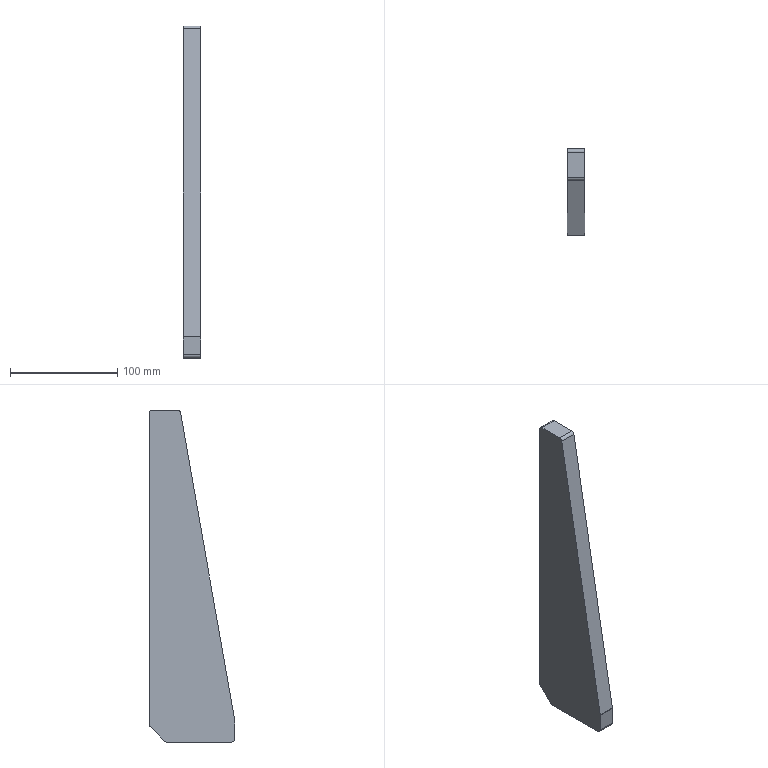Part | STEP file | SN10_006_005-03_REFORCO | 1 solid | 14 faces | box 16 x 80 x 310 mm | volume 276279 mm3 | plane 8 | cylinder 6 | commonest cylinder face diameters 6 x6
STEP:
#1=CARTESIAN_POINT('',(0.,0.,0.));
#2=DIRECTION('',(0.,0.,1.));
#3=DIRECTION('',(1.,0.,0.));
#4=AXIS2_PLACEMENT_3D('',#1,#2,#3);
#5=CARTESIAN_POINT('',(233.,-222.348,383.5));
#6=VERTEX_POINT('',#5);
#7=CARTESIAN_POINT('',(233.,-225.302,381.021));
#8=VERTEX_POINT('',#7);
#9=CARTESIAN_POINT('',(233.,-222.348,380.5));
#10=DIRECTION('',(1.,0.,0.));
#11=DIRECTION('',(0.,1.,0.));
#12=AXIS2_PLACEMENT_3D('',#9,#10,#11);
#13=CIRCLE('',#12,3.);
#14=CARTESIAN_POINT('',(225.,-222.348,380.5));
#15=DIRECTION('',(1.,0.,0.));
#16=DIRECTION('',(0.,0.,1.));
#17=AXIS2_PLACEMENT_3D('',#14,#15,#16);
#18=CYLINDRICAL_SURFACE('',#17,3.);
#19=CARTESIAN_POINT('',(-1.571,8.));
#20=DIRECTION('',(1.,0.));
#21=VECTOR('',#20,1.);
#22=LINE('',#19,#21);
#23=(GEOMETRIC_REPRESENTATION_CONTEXT(2)PARAMETRIC_REPRESENTATION_CONTEXT()REPRESENTATION_CONTEXT('',''));
#24=DEFINITIONAL_REPRESENTATION('',(#22),#23);
#25=PCURVE('',#18,#24);
#26=CARTESIAN_POINT('',(233.,-276.,73.5));
#27=DIRECTION('',(-1.,0.,0.));
#28=DIRECTION('',(0.,0.,1.));
#29=AXIS2_PLACEMENT_3D('',#26,#27,#28);
#30=PLANE('',#29);
#31=CARTESIAN_POINT('',(307.,56.652));
#32=CARTESIAN_POINT('',(312.196,56.652));
#33=CARTESIAN_POINT('',(309.598,52.152));
#34=CARTESIAN_POINT('',(307.,47.652));
#35=CARTESIAN_POINT('',(304.402,52.152));
#36=CARTESIAN_POINT('',(301.804,56.652));
#37=CARTESIAN_POINT('',(307.,56.652));
#38=(BOUNDED_CURVE()B_SPLINE_CURVE(2,(#31,#32,#33,#34,#35,#36,#37),.UNSPECIFIED.,.T.,.F.)B_SPLINE_CURVE_WITH_KNOTS((1,2,2,2,2,1),(-2.094,0.,2.094,4.189,6.283,8.378),.UNSPECIFIED.)CURVE()GEOMETRIC_REPRESENTATION_ITEM()RATIONAL_B_SPLINE_CURVE((1.,0.5,1.,0.5,1.,0.5,1.))REPRESENTATION_ITEM(''));
#39=(GEOMETRIC_REPRESENTATION_CONTEXT(2)PARAMETRIC_REPRESENTATION_CONTEXT()REPRESENTATION_CONTEXT('',''));
#40=DEFINITIONAL_REPRESENTATION('',(#38),#39);
#41=PCURVE('',#30,#40);
#42=SURFACE_CURVE('',#13,(#25,#41),.PCURVE_S1.);
#43=EDGE_CURVE('',#6,#8,#42,.T.);
#44=ORIENTED_EDGE('',*,*,#43,.F.);
#45=CARTESIAN_POINT('',(217.,-222.348,383.5));
#46=VERTEX_POINT('',#45);
#47=CARTESIAN_POINT('',(217.,-222.348,383.5));
#48=DIRECTION('',(1.,0.,0.));
#49=VECTOR('',#48,1.);
#50=LINE('',#47,#49);
#51=CARTESIAN_POINT('',(0.,-8.));
#52=DIRECTION('',(0.,1.));
#53=VECTOR('',#52,1.);
#54=LINE('',#51,#53);
#55=(GEOMETRIC_REPRESENTATION_CONTEXT(2)PARAMETRIC_REPRESENTATION_CONTEXT()REPRESENTATION_CONTEXT('',''));
#56=DEFINITIONAL_REPRESENTATION('',(#54),#55);
#57=PCURVE('',#18,#56);
#58=CARTESIAN_POINT('',(200.,-224.865,383.5));
#59=DIRECTION('',(0.,0.,-1.));
#60=DIRECTION('',(-1.,0.,0.));
#61=AXIS2_PLACEMENT_3D('',#58,#59,#60);
#62=PLANE('',#61);
#63=CARTESIAN_POINT('',(-17.,2.517));
#64=DIRECTION('',(-1.,0.));
#65=VECTOR('',#64,1.);
#66=LINE('',#63,#65);
#67=(GEOMETRIC_REPRESENTATION_CONTEXT(2)PARAMETRIC_REPRESENTATION_CONTEXT()REPRESENTATION_CONTEXT('',''));
#68=DEFINITIONAL_REPRESENTATION('',(#66),#67);
#69=PCURVE('',#62,#68);
#70=SURFACE_CURVE('',#50,(#57,#69),.PCURVE_S1.);
#71=EDGE_CURVE('',#46,#6,#70,.T.);
#72=ORIENTED_EDGE('',*,*,#71,.F.);
#73=CARTESIAN_POINT('',(217.,-225.302,381.021));
#74=VERTEX_POINT('',#73);
#75=CARTESIAN_POINT('',(217.,-222.348,380.5));
#76=DIRECTION('',(1.,0.,0.));
#77=DIRECTION('',(0.,1.,0.));
#78=AXIS2_PLACEMENT_3D('',#75,#76,#77);
#79=CIRCLE('',#78,3.);
#80=CARTESIAN_POINT('',(-1.571,-8.));
#81=DIRECTION('',(1.,0.));
#82=VECTOR('',#81,1.);
#83=LINE('',#80,#82);
#84=(GEOMETRIC_REPRESENTATION_CONTEXT(2)PARAMETRIC_REPRESENTATION_CONTEXT()REPRESENTATION_CONTEXT('',''));
#85=DEFINITIONAL_REPRESENTATION('',(#83),#84);
#86=PCURVE('',#18,#85);
#87=CARTESIAN_POINT('',(217.,-276.,383.5));
#88=DIRECTION('',(1.,0.,0.));
#89=DIRECTION('',(0.,0.,-1.));
#90=AXIS2_PLACEMENT_3D('',#87,#88,#89);
#91=PLANE('',#90);
#92=CARTESIAN_POINT('',(3.,53.652));
#93=DIRECTION('',(0.,1.));
#94=AXIS2_PLACEMENT_2D('',#92,#93);
#95=CIRCLE('',#94,3.);
#96=(GEOMETRIC_REPRESENTATION_CONTEXT(2)PARAMETRIC_REPRESENTATION_CONTEXT()REPRESENTATION_CONTEXT('',''));
#97=DEFINITIONAL_REPRESENTATION('',(#95),#96);
#98=PCURVE('',#91,#97);
#99=SURFACE_CURVE('',#79,(#86,#98),.PCURVE_S1.);
#100=EDGE_CURVE('',#46,#74,#99,.T.);
#101=ORIENTED_EDGE('',*,*,#100,.T.);
#102=CARTESIAN_POINT('',(217.,-225.302,381.021));
#103=DIRECTION('',(1.,0.,0.));
#104=VECTOR('',#103,1.);
#105=LINE('',#102,#104);
#106=CARTESIAN_POINT('',(1.396,-8.));
#107=DIRECTION('',(0.,1.));
#108=VECTOR('',#107,1.);
#109=LINE('',#106,#108);
#110=(GEOMETRIC_REPRESENTATION_CONTEXT(2)PARAMETRIC_REPRESENTATION_CONTEXT()REPRESENTATION_CONTEXT('',''));
#111=DEFINITIONAL_REPRESENTATION('',(#109),#110);
#112=PCURVE('',#18,#111);
#113=CARTESIAN_POINT('',(200.,-276.,93.5));
#114=DIRECTION('',(0.,0.9848,-0.1736));
#115=DIRECTION('',(0.,0.1736,0.9848));
#116=AXIS2_PLACEMENT_3D('',#113,#114,#115);
#117=PLANE('',#116);
#118=CARTESIAN_POINT('',(291.956,17.));
#119=DIRECTION('',(0.,1.));
#120=VECTOR('',#119,1.);
#121=LINE('',#118,#120);
#122=(GEOMETRIC_REPRESENTATION_CONTEXT(2)PARAMETRIC_REPRESENTATION_CONTEXT()REPRESENTATION_CONTEXT('',''));
#123=DEFINITIONAL_REPRESENTATION('',(#121),#122);
#124=PCURVE('',#117,#123);
#125=SURFACE_CURVE('',#105,(#112,#124),.PCURVE_S1.);
#126=EDGE_CURVE('',#74,#8,#125,.T.);
#127=ORIENTED_EDGE('',*,*,#126,.T.);
#128=EDGE_LOOP('',(#44,#72,#101,#127));
#129=FACE_BOUND('',#128,.T.);
#130=ADVANCED_FACE('',(#129),#18,.T.);
#131=CARTESIAN_POINT('',(217.,-275.954,93.758));
#132=VERTEX_POINT('',#131);
#133=CARTESIAN_POINT('',(233.,-275.954,93.758));
#134=VERTEX_POINT('',#133);
#135=CARTESIAN_POINT('',(217.,-275.954,93.758));
#136=DIRECTION('',(1.,0.,0.));
#137=VECTOR('',#136,1.);
#138=LINE('',#135,#137);
#139=CARTESIAN_POINT('',(0.2625,17.));
#140=DIRECTION('',(0.,1.));
#141=VECTOR('',#140,1.);
#142=LINE('',#139,#141);
#143=(GEOMETRIC_REPRESENTATION_CONTEXT(2)PARAMETRIC_REPRESENTATION_CONTEXT()REPRESENTATION_CONTEXT('',''));
#144=DEFINITIONAL_REPRESENTATION('',(#142),#143);
#145=PCURVE('',#117,#144);
#146=CARTESIAN_POINT('',(225.,-273.,93.238));
#147=DIRECTION('',(1.,0.,0.));
#148=DIRECTION('',(0.,-0.9848,0.1736));
#149=AXIS2_PLACEMENT_3D('',#146,#147,#148);
#150=CYLINDRICAL_SURFACE('',#149,3.);
#151=CARTESIAN_POINT('',(0.,-8.));
#152=DIRECTION('',(0.,1.));
#153=VECTOR('',#152,1.);
#154=LINE('',#151,#153);
#155=(GEOMETRIC_REPRESENTATION_CONTEXT(2)PARAMETRIC_REPRESENTATION_CONTEXT()REPRESENTATION_CONTEXT('',''));
#156=DEFINITIONAL_REPRESENTATION('',(#154),#155);
#157=PCURVE('',#150,#156);
#158=SURFACE_CURVE('',#138,(#145,#157),.PCURVE_S1.);
#159=EDGE_CURVE('',#132,#134,#158,.T.);
#160=ORIENTED_EDGE('',*,*,#159,.T.);
#161=CARTESIAN_POINT('',(233.,-225.302,381.021));
#162=DIRECTION('',(0.,-0.1736,-0.9848));
#163=VECTOR('',#162,1.);
#164=LINE('',#161,#163);
#165=CARTESIAN_POINT('',(291.956,33.));
#166=DIRECTION('',(-1.,0.));
#167=VECTOR('',#166,1.);
#168=LINE('',#165,#167);
#169=(GEOMETRIC_REPRESENTATION_CONTEXT(2)PARAMETRIC_REPRESENTATION_CONTEXT()REPRESENTATION_CONTEXT('',''));
#170=DEFINITIONAL_REPRESENTATION('',(#168),#169);
#171=PCURVE('',#117,#170);
#172=CARTESIAN_POINT('',(307.521,50.698));
#173=DIRECTION('',(-0.9848,-0.1736));
#174=VECTOR('',#173,1.);
#175=LINE('',#172,#174);
#176=(GEOMETRIC_REPRESENTATION_CONTEXT(2)PARAMETRIC_REPRESENTATION_CONTEXT()REPRESENTATION_CONTEXT('',''));
#177=DEFINITIONAL_REPRESENTATION('',(#175),#176);
#178=PCURVE('',#30,#177);
#179=SURFACE_CURVE('',#164,(#171,#178),.PCURVE_S1.);
#180=EDGE_CURVE('',#8,#134,#179,.T.);
#181=ORIENTED_EDGE('',*,*,#180,.F.);
#182=ORIENTED_EDGE('',*,*,#126,.F.);
#183=CARTESIAN_POINT('',(217.,-225.302,381.021));
#184=DIRECTION('',(0.,-0.1736,-0.9848));
#185=VECTOR('',#184,1.);
#186=LINE('',#183,#185);
#187=CARTESIAN_POINT('',(291.956,17.));
#188=DIRECTION('',(-1.,0.));
#189=VECTOR('',#188,1.);
#190=LINE('',#187,#189);
#191=(GEOMETRIC_REPRESENTATION_CONTEXT(2)PARAMETRIC_REPRESENTATION_CONTEXT()REPRESENTATION_CONTEXT('',''));
#192=DEFINITIONAL_REPRESENTATION('',(#190),#191);
#193=PCURVE('',#117,#192);
#194=CARTESIAN_POINT('',(2.479,50.698));
#195=DIRECTION('',(0.9848,-0.1736));
#196=VECTOR('',#195,1.);
#197=LINE('',#194,#196);
#198=(GEOMETRIC_REPRESENTATION_CONTEXT(2)PARAMETRIC_REPRESENTATION_CONTEXT()REPRESENTATION_CONTEXT('',''));
#199=DEFINITIONAL_REPRESENTATION('',(#197),#198);
#200=PCURVE('',#91,#199);
#201=SURFACE_CURVE('',#186,(#193,#200),.PCURVE_S1.);
#202=EDGE_CURVE('',#74,#132,#201,.T.);
#203=ORIENTED_EDGE('',*,*,#202,.T.);
#204=EDGE_LOOP('',(#160,#181,#182,#203));
#205=FACE_BOUND('',#204,.T.);
#206=ADVANCED_FACE('',(#205),#117,.F.);
#207=CARTESIAN_POINT('',(233.,-276.,93.238));
#208=VERTEX_POINT('',#207);
#209=CARTESIAN_POINT('',(233.,-273.,93.238));
#210=DIRECTION('',(1.,0.,0.));
#211=DIRECTION('',(0.,1.,0.));
#212=AXIS2_PLACEMENT_3D('',#209,#210,#211);
#213=CIRCLE('',#212,3.);
#214=CARTESIAN_POINT('',(-2.967,8.));
#215=DIRECTION('',(1.,0.));
#216=VECTOR('',#215,1.);
#217=LINE('',#214,#216);
#218=(GEOMETRIC_REPRESENTATION_CONTEXT(2)PARAMETRIC_REPRESENTATION_CONTEXT()REPRESENTATION_CONTEXT('',''));
#219=DEFINITIONAL_REPRESENTATION('',(#217),#218);
#220=PCURVE('',#150,#219);
#221=CARTESIAN_POINT('',(19.738,6.));
#222=CARTESIAN_POINT('',(24.934,6.));
#223=CARTESIAN_POINT('',(22.336,1.5));
#224=CARTESIAN_POINT('',(19.738,-3.));
#225=CARTESIAN_POINT('',(17.139,1.5));
#226=CARTESIAN_POINT('',(14.541,6.));
#227=CARTESIAN_POINT('',(19.738,6.));
#228=(BOUNDED_CURVE()B_SPLINE_CURVE(2,(#221,#222,#223,#224,#225,#226,#227),.UNSPECIFIED.,.T.,.F.)B_SPLINE_CURVE_WITH_KNOTS((1,2,2,2,2,1),(-2.094,0.,2.094,4.189,6.283,8.378),.UNSPECIFIED.)CURVE()GEOMETRIC_REPRESENTATION_ITEM()RATIONAL_B_SPLINE_CURVE((1.,0.5,1.,0.5,1.,0.5,1.))REPRESENTATION_ITEM(''));
#229=(GEOMETRIC_REPRESENTATION_CONTEXT(2)PARAMETRIC_REPRESENTATION_CONTEXT()REPRESENTATION_CONTEXT('',''));
#230=DEFINITIONAL_REPRESENTATION('',(#228),#229);
#231=PCURVE('',#30,#230);
#232=SURFACE_CURVE('',#213,(#220,#231),.PCURVE_S1.);
#233=EDGE_CURVE('',#134,#208,#232,.T.);
#234=ORIENTED_EDGE('',*,*,#233,.F.);
#235=ORIENTED_EDGE('',*,*,#159,.F.);
#236=CARTESIAN_POINT('',(217.,-276.,93.238));
#237=VERTEX_POINT('',#236);
#238=CARTESIAN_POINT('',(217.,-273.,93.238));
#239=DIRECTION('',(1.,0.,0.));
#240=DIRECTION('',(0.,1.,0.));
#241=AXIS2_PLACEMENT_3D('',#238,#239,#240);
#242=CIRCLE('',#241,3.);
#243=CARTESIAN_POINT('',(-2.967,-8.));
#244=DIRECTION('',(1.,0.));
#245=VECTOR('',#244,1.);
#246=LINE('',#243,#245);
#247=(GEOMETRIC_REPRESENTATION_CONTEXT(2)PARAMETRIC_REPRESENTATION_CONTEXT()REPRESENTATION_CONTEXT('',''));
#248=DEFINITIONAL_REPRESENTATION('',(#246),#247);
#249=PCURVE('',#150,#248);
#250=CARTESIAN_POINT('',(290.262,3.));
#251=DIRECTION('',(0.,1.));
#252=AXIS2_PLACEMENT_2D('',#250,#251);
#253=CIRCLE('',#252,3.);
#254=(GEOMETRIC_REPRESENTATION_CONTEXT(2)PARAMETRIC_REPRESENTATION_CONTEXT()REPRESENTATION_CONTEXT('',''));
#255=DEFINITIONAL_REPRESENTATION('',(#253),#254);
#256=PCURVE('',#91,#255);
#257=SURFACE_CURVE('',#242,(#249,#256),.PCURVE_S1.);
#258=EDGE_CURVE('',#132,#237,#257,.T.);
#259=ORIENTED_EDGE('',*,*,#258,.T.);
#260=CARTESIAN_POINT('',(217.,-276.,93.238));
#261=DIRECTION('',(1.,0.,0.));
#262=VECTOR('',#261,1.);
#263=LINE('',#260,#262);
#264=CARTESIAN_POINT('',(0.1745,-8.));
#265=DIRECTION('',(0.,1.));
#266=VECTOR('',#265,1.);
#267=LINE('',#264,#266);
#268=(GEOMETRIC_REPRESENTATION_CONTEXT(2)PARAMETRIC_REPRESENTATION_CONTEXT()REPRESENTATION_CONTEXT('',''));
#269=DEFINITIONAL_REPRESENTATION('',(#267),#268);
#270=PCURVE('',#150,#269);
#271=CARTESIAN_POINT('',(200.,-276.,73.5));
#272=DIRECTION('',(0.,1.,0.));
#273=DIRECTION('',(0.,0.,1.));
#274=AXIS2_PLACEMENT_3D('',#271,#272,#273);
#275=PLANE('',#274);
#276=CARTESIAN_POINT('',(19.738,17.));
#277=DIRECTION('',(0.,1.));
#278=VECTOR('',#277,1.);
#279=LINE('',#276,#278);
#280=(GEOMETRIC_REPRESENTATION_CONTEXT(2)PARAMETRIC_REPRESENTATION_CONTEXT()REPRESENTATION_CONTEXT('',''));
#281=DEFINITIONAL_REPRESENTATION('',(#279),#280);
#282=PCURVE('',#275,#281);
#283=SURFACE_CURVE('',#263,(#270,#282),.PCURVE_S1.);
#284=EDGE_CURVE('',#237,#208,#283,.T.);
#285=ORIENTED_EDGE('',*,*,#284,.T.);
#286=EDGE_LOOP('',(#234,#235,#259,#285));
#287=FACE_BOUND('',#286,.T.);
#288=ADVANCED_FACE('',(#287),#150,.T.);
#289=CARTESIAN_POINT('',(217.,-276.,76.5));
#290=VERTEX_POINT('',#289);
#291=CARTESIAN_POINT('',(233.,-276.,76.5));
#292=VERTEX_POINT('',#291);
#293=CARTESIAN_POINT('',(217.,-276.,76.5));
#294=DIRECTION('',(1.,0.,0.));
#295=VECTOR('',#294,1.);
#296=LINE('',#293,#295);
#297=CARTESIAN_POINT('',(3.,17.));
#298=DIRECTION('',(0.,1.));
#299=VECTOR('',#298,1.);
#300=LINE('',#297,#299);
#301=(GEOMETRIC_REPRESENTATION_CONTEXT(2)PARAMETRIC_REPRESENTATION_CONTEXT()REPRESENTATION_CONTEXT('',''));
#302=DEFINITIONAL_REPRESENTATION('',(#300),#301);
#303=PCURVE('',#275,#302);
#304=CARTESIAN_POINT('',(225.,-273.,76.5));
#305=DIRECTION('',(1.,0.,0.));
#306=DIRECTION('',(0.,-1.,0.));
#307=AXIS2_PLACEMENT_3D('',#304,#305,#306);
#308=CYLINDRICAL_SURFACE('',#307,3.);
#309=CARTESIAN_POINT('',(0.,-8.));
#310=DIRECTION('',(0.,1.));
#311=VECTOR('',#310,1.);
#312=LINE('',#309,#311);
#313=(GEOMETRIC_REPRESENTATION_CONTEXT(2)PARAMETRIC_REPRESENTATION_CONTEXT()REPRESENTATION_CONTEXT('',''));
#314=DEFINITIONAL_REPRESENTATION('',(#312),#313);
#315=PCURVE('',#308,#314);
#316=SURFACE_CURVE('',#296,(#303,#315),.PCURVE_S1.);
#317=EDGE_CURVE('',#290,#292,#316,.T.);
#318=ORIENTED_EDGE('',*,*,#317,.T.);
#319=CARTESIAN_POINT('',(233.,-276.,76.5));
#320=DIRECTION('',(0.,0.,1.));
#321=VECTOR('',#320,1.);
#322=LINE('',#319,#321);
#323=CARTESIAN_POINT('',(3.,33.));
#324=DIRECTION('',(1.,0.));
#325=VECTOR('',#324,1.);
#326=LINE('',#323,#325);
#327=(GEOMETRIC_REPRESENTATION_CONTEXT(2)PARAMETRIC_REPRESENTATION_CONTEXT()REPRESENTATION_CONTEXT('',''));
#328=DEFINITIONAL_REPRESENTATION('',(#326),#327);
#329=PCURVE('',#275,#328);
#330=CARTESIAN_POINT('',(3.,0.));
#331=DIRECTION('',(1.,0.));
#332=VECTOR('',#331,1.);
#333=LINE('',#330,#332);
#334=(GEOMETRIC_REPRESENTATION_CONTEXT(2)PARAMETRIC_REPRESENTATION_CONTEXT()REPRESENTATION_CONTEXT('',''));
#335=DEFINITIONAL_REPRESENTATION('',(#333),#334);
#336=PCURVE('',#30,#335);
#337=SURFACE_CURVE('',#322,(#329,#336),.PCURVE_S1.);
#338=EDGE_CURVE('',#292,#208,#337,.T.);
#339=ORIENTED_EDGE('',*,*,#338,.T.);
#340=ORIENTED_EDGE('',*,*,#284,.F.);
#341=CARTESIAN_POINT('',(217.,-276.,93.238));
#342=DIRECTION('',(0.,0.,-1.));
#343=VECTOR('',#342,1.);
#344=LINE('',#341,#343);
#345=CARTESIAN_POINT('',(19.738,17.));
#346=DIRECTION('',(-1.,0.));
#347=VECTOR('',#346,1.);
#348=LINE('',#345,#347);
#349=(GEOMETRIC_REPRESENTATION_CONTEXT(2)PARAMETRIC_REPRESENTATION_CONTEXT()REPRESENTATION_CONTEXT('',''));
#350=DEFINITIONAL_REPRESENTATION('',(#348),#349);
#351=PCURVE('',#275,#350);
#352=CARTESIAN_POINT('',(290.262,0.));
#353=DIRECTION('',(1.,0.));
#354=VECTOR('',#353,1.);
#355=LINE('',#352,#354);
#356=(GEOMETRIC_REPRESENTATION_CONTEXT(2)PARAMETRIC_REPRESENTATION_CONTEXT()REPRESENTATION_CONTEXT('',''));
#357=DEFINITIONAL_REPRESENTATION('',(#355),#356);
#358=PCURVE('',#91,#357);
#359=SURFACE_CURVE('',#344,(#351,#358),.PCURVE_S1.);
#360=EDGE_CURVE('',#237,#290,#359,.T.);
#361=ORIENTED_EDGE('',*,*,#360,.T.);
#362=EDGE_LOOP('',(#318,#339,#340,#361));
#363=FACE_BOUND('',#362,.T.);
#364=ADVANCED_FACE('',(#363),#275,.F.);
#365=CARTESIAN_POINT('',(233.,-273.,73.5));
#366=VERTEX_POINT('',#365);
#367=CARTESIAN_POINT('',(233.,-273.,76.5));
#368=DIRECTION('',(1.,0.,0.));
#369=DIRECTION('',(0.,1.,0.));
#370=AXIS2_PLACEMENT_3D('',#367,#368,#369);
#371=CIRCLE('',#370,3.);
#372=CARTESIAN_POINT('',(-3.142,8.));
#373=DIRECTION('',(1.,0.));
#374=VECTOR('',#373,1.);
#375=LINE('',#372,#374);
#376=(GEOMETRIC_REPRESENTATION_CONTEXT(2)PARAMETRIC_REPRESENTATION_CONTEXT()REPRESENTATION_CONTEXT('',''));
#377=DEFINITIONAL_REPRESENTATION('',(#375),#376);
#378=PCURVE('',#308,#377);
#379=CARTESIAN_POINT('',(3.,6.));
#380=CARTESIAN_POINT('',(8.196,6.));
#381=CARTESIAN_POINT('',(5.598,1.5));
#382=CARTESIAN_POINT('',(3.,-3.));
#383=CARTESIAN_POINT('',(0.4019,1.5));
#384=CARTESIAN_POINT('',(-2.196,6.));
#385=CARTESIAN_POINT('',(3.,6.));
#386=(BOUNDED_CURVE()B_SPLINE_CURVE(2,(#379,#380,#381,#382,#383,#384,#385),.UNSPECIFIED.,.T.,.F.)B_SPLINE_CURVE_WITH_KNOTS((1,2,2,2,2,1),(-2.094,0.,2.094,4.189,6.283,8.378),.UNSPECIFIED.)CURVE()GEOMETRIC_REPRESENTATION_ITEM()RATIONAL_B_SPLINE_CURVE((1.,0.5,1.,0.5,1.,0.5,1.))REPRESENTATION_ITEM(''));
#387=(GEOMETRIC_REPRESENTATION_CONTEXT(2)PARAMETRIC_REPRESENTATION_CONTEXT()REPRESENTATION_CONTEXT('',''));
#388=DEFINITIONAL_REPRESENTATION('',(#386),#387);
#389=PCURVE('',#30,#388);
#390=SURFACE_CURVE('',#371,(#378,#389),.PCURVE_S1.);
#391=EDGE_CURVE('',#292,#366,#390,.T.);
#392=ORIENTED_EDGE('',*,*,#391,.F.);
#393=ORIENTED_EDGE('',*,*,#317,.F.);
#394=CARTESIAN_POINT('',(217.,-273.,73.5));
#395=VERTEX_POINT('',#394);
#396=CARTESIAN_POINT('',(217.,-273.,76.5));
#397=DIRECTION('',(1.,0.,0.));
#398=DIRECTION('',(0.,1.,0.));
#399=AXIS2_PLACEMENT_3D('',#396,#397,#398);
#400=CIRCLE('',#399,3.);
#401=CARTESIAN_POINT('',(-3.142,-8.));
#402=DIRECTION('',(1.,0.));
#403=VECTOR('',#402,1.);
#404=LINE('',#401,#403);
#405=(GEOMETRIC_REPRESENTATION_CONTEXT(2)PARAMETRIC_REPRESENTATION_CONTEXT()REPRESENTATION_CONTEXT('',''));
#406=DEFINITIONAL_REPRESENTATION('',(#404),#405);
#407=PCURVE('',#308,#406);
#408=CARTESIAN_POINT('',(307.,3.));
#409=DIRECTION('',(0.,1.));
#410=AXIS2_PLACEMENT_2D('',#408,#409);
#411=CIRCLE('',#410,3.);
#412=(GEOMETRIC_REPRESENTATION_CONTEXT(2)PARAMETRIC_REPRESENTATION_CONTEXT()REPRESENTATION_CONTEXT('',''));
#413=DEFINITIONAL_REPRESENTATION('',(#411),#412);
#414=PCURVE('',#91,#413);
#415=SURFACE_CURVE('',#400,(#407,#414),.PCURVE_S1.);
#416=EDGE_CURVE('',#290,#395,#415,.T.);
#417=ORIENTED_EDGE('',*,*,#416,.T.);
#418=CARTESIAN_POINT('',(217.,-273.,73.5));
#419=DIRECTION('',(1.,0.,0.));
#420=VECTOR('',#419,1.);
#421=LINE('',#418,#420);
#422=CARTESIAN_POINT('',(1.571,-8.));
#423=DIRECTION('',(0.,1.));
#424=VECTOR('',#423,1.);
#425=LINE('',#422,#424);
#426=(GEOMETRIC_REPRESENTATION_CONTEXT(2)PARAMETRIC_REPRESENTATION_CONTEXT()REPRESENTATION_CONTEXT('',''));
#427=DEFINITIONAL_REPRESENTATION('',(#425),#426);
#428=PCURVE('',#308,#427);
#429=CARTESIAN_POINT('',(200.,-211.,73.5));
#430=DIRECTION('',(0.,0.,1.));
#431=DIRECTION('',(1.,0.,0.));
#432=AXIS2_PLACEMENT_3D('',#429,#430,#431);
#433=PLANE('',#432);
#434=CARTESIAN_POINT('',(17.,-62.));
#435=DIRECTION('',(1.,0.));
#436=VECTOR('',#435,1.);
#437=LINE('',#434,#436);
#438=(GEOMETRIC_REPRESENTATION_CONTEXT(2)PARAMETRIC_REPRESENTATION_CONTEXT()REPRESENTATION_CONTEXT('',''));
#439=DEFINITIONAL_REPRESENTATION('',(#437),#438);
#440=PCURVE('',#433,#439);
#441=SURFACE_CURVE('',#421,(#428,#440),.PCURVE_S1.);
#442=EDGE_CURVE('',#395,#366,#441,.T.);
#443=ORIENTED_EDGE('',*,*,#442,.T.);
#444=EDGE_LOOP('',(#392,#393,#417,#443));
#445=FACE_BOUND('',#444,.T.);
#446=ADVANCED_FACE('',(#445),#308,.T.);
#447=CARTESIAN_POINT('',(217.,-212.243,73.5));
#448=VERTEX_POINT('',#447);
#449=CARTESIAN_POINT('',(233.,-212.243,73.5));
#450=VERTEX_POINT('',#449);
#451=CARTESIAN_POINT('',(217.,-212.243,73.5));
#452=DIRECTION('',(1.,0.,0.));
#453=VECTOR('',#452,1.);
#454=LINE('',#451,#453);
#455=CARTESIAN_POINT('',(17.,-1.243));
#456=DIRECTION('',(1.,0.));
#457=VECTOR('',#456,1.);
#458=LINE('',#455,#457);
#459=(GEOMETRIC_REPRESENTATION_CONTEXT(2)PARAMETRIC_REPRESENTATION_CONTEXT()REPRESENTATION_CONTEXT('',''));
#460=DEFINITIONAL_REPRESENTATION('',(#458),#459);
#461=PCURVE('',#433,#460);
#462=CARTESIAN_POINT('',(225.,-212.243,76.5));
#463=DIRECTION('',(1.,0.,0.));
#464=DIRECTION('',(0.,0.,-1.));
#465=AXIS2_PLACEMENT_3D('',#462,#463,#464);
#466=CYLINDRICAL_SURFACE('',#465,3.);
#467=CARTESIAN_POINT('',(0.,-8.));
#468=DIRECTION('',(0.,1.));
#469=VECTOR('',#468,1.);
#470=LINE('',#467,#469);
#471=(GEOMETRIC_REPRESENTATION_CONTEXT(2)PARAMETRIC_REPRESENTATION_CONTEXT()REPRESENTATION_CONTEXT('',''));
#472=DEFINITIONAL_REPRESENTATION('',(#470),#471);
#473=PCURVE('',#466,#472);
#474=SURFACE_CURVE('',#454,(#461,#473),.PCURVE_S1.);
#475=EDGE_CURVE('',#448,#450,#474,.T.);
#476=ORIENTED_EDGE('',*,*,#475,.T.);
#477=CARTESIAN_POINT('',(233.,-273.,73.5));
#478=DIRECTION('',(0.,1.,0.));
#479=VECTOR('',#478,1.);
#480=LINE('',#477,#479);
#481=CARTESIAN_POINT('',(33.,-62.));
#482=DIRECTION('',(0.,1.));
#483=VECTOR('',#482,1.);
#484=LINE('',#481,#483);
#485=(GEOMETRIC_REPRESENTATION_CONTEXT(2)PARAMETRIC_REPRESENTATION_CONTEXT()REPRESENTATION_CONTEXT('',''));
#486=DEFINITIONAL_REPRESENTATION('',(#484),#485);
#487=PCURVE('',#433,#486);
#488=CARTESIAN_POINT('',(0.,3.));
#489=DIRECTION('',(0.,1.));
#490=VECTOR('',#489,1.);
#491=LINE('',#488,#490);
#492=(GEOMETRIC_REPRESENTATION_CONTEXT(2)PARAMETRIC_REPRESENTATION_CONTEXT()REPRESENTATION_CONTEXT('',''));
#493=DEFINITIONAL_REPRESENTATION('',(#491),#492);
#494=PCURVE('',#30,#493);
#495=SURFACE_CURVE('',#480,(#487,#494),.PCURVE_S1.);
#496=EDGE_CURVE('',#366,#450,#495,.T.);
#497=ORIENTED_EDGE('',*,*,#496,.F.);
#498=ORIENTED_EDGE('',*,*,#442,.F.);
#499=CARTESIAN_POINT('',(217.,-273.,73.5));
#500=DIRECTION('',(0.,1.,0.));
#501=VECTOR('',#500,1.);
#502=LINE('',#499,#501);
#503=CARTESIAN_POINT('',(17.,-62.));
#504=DIRECTION('',(0.,1.));
#505=VECTOR('',#504,1.);
#506=LINE('',#503,#505);
#507=(GEOMETRIC_REPRESENTATION_CONTEXT(2)PARAMETRIC_REPRESENTATION_CONTEXT()REPRESENTATION_CONTEXT('',''));
#508=DEFINITIONAL_REPRESENTATION('',(#506),#507);
#509=PCURVE('',#433,#508);
#510=CARTESIAN_POINT('',(310.,3.));
#511=DIRECTION('',(0.,1.));
#512=VECTOR('',#511,1.);
#513=LINE('',#510,#512);
#514=(GEOMETRIC_REPRESENTATION_CONTEXT(2)PARAMETRIC_REPRESENTATION_CONTEXT()REPRESENTATION_CONTEXT('',''));
#515=DEFINITIONAL_REPRESENTATION('',(#513),#514);
#516=PCURVE('',#91,#515);
#517=SURFACE_CURVE('',#502,(#509,#516),.PCURVE_S1.);
#518=EDGE_CURVE('',#395,#448,#517,.T.);
#519=ORIENTED_EDGE('',*,*,#518,.T.);
#520=EDGE_LOOP('',(#476,#497,#498,#519));
#521=FACE_BOUND('',#520,.T.);
#522=ADVANCED_FACE('',(#521),#433,.F.);
#523=CARTESIAN_POINT('',(233.,-210.121,74.379));
#524=VERTEX_POINT('',#523);
#525=CARTESIAN_POINT('',(233.,-212.243,76.5));
#526=DIRECTION('',(1.,0.,0.));
#527=DIRECTION('',(0.,1.,0.));
#528=AXIS2_PLACEMENT_3D('',#525,#526,#527);
#529=CIRCLE('',#528,3.);
#530=CARTESIAN_POINT('',(-4.712,8.));
#531=DIRECTION('',(1.,0.));
#532=VECTOR('',#531,1.);
#533=LINE('',#530,#532);
#534=(GEOMETRIC_REPRESENTATION_CONTEXT(2)PARAMETRIC_REPRESENTATION_CONTEXT()REPRESENTATION_CONTEXT('',''));
#535=DEFINITIONAL_REPRESENTATION('',(#533),#534);
#536=PCURVE('',#466,#535);
#537=CARTESIAN_POINT('',(3.,66.757));
#538=CARTESIAN_POINT('',(8.196,66.757));
#539=CARTESIAN_POINT('',(5.598,62.257));
#540=CARTESIAN_POINT('',(3.,57.757));
#541=CARTESIAN_POINT('',(0.4019,62.257));
#542=CARTESIAN_POINT('',(-2.196,66.757));
#543=CARTESIAN_POINT('',(3.,66.757));
#544=(BOUNDED_CURVE()B_SPLINE_CURVE(2,(#537,#538,#539,#540,#541,#542,#543),.UNSPECIFIED.,.T.,.F.)B_SPLINE_CURVE_WITH_KNOTS((1,2,2,2,2,1),(-2.094,0.,2.094,4.189,6.283,8.378),.UNSPECIFIED.)CURVE()GEOMETRIC_REPRESENTATION_ITEM()RATIONAL_B_SPLINE_CURVE((1.,0.5,1.,0.5,1.,0.5,1.))REPRESENTATION_ITEM(''));
#545=(GEOMETRIC_REPRESENTATION_CONTEXT(2)PARAMETRIC_REPRESENTATION_CONTEXT()REPRESENTATION_CONTEXT('',''));
#546=DEFINITIONAL_REPRESENTATION('',(#544),#545);
#547=PCURVE('',#30,#546);
#548=SURFACE_CURVE('',#529,(#536,#547),.PCURVE_S1.);
#549=EDGE_CURVE('',#450,#524,#548,.T.);
#550=ORIENTED_EDGE('',*,*,#549,.F.);
#551=ORIENTED_EDGE('',*,*,#475,.F.);
#552=CARTESIAN_POINT('',(217.,-210.121,74.379));
#553=VERTEX_POINT('',#552);
#554=CARTESIAN_POINT('',(217.,-212.243,76.5));
#555=DIRECTION('',(1.,0.,0.));
#556=DIRECTION('',(0.,1.,0.));
#557=AXIS2_PLACEMENT_3D('',#554,#555,#556);
#558=CIRCLE('',#557,3.);
#559=CARTESIAN_POINT('',(-4.712,-8.));
#560=DIRECTION('',(1.,0.));
#561=VECTOR('',#560,1.);
#562=LINE('',#559,#561);
#563=(GEOMETRIC_REPRESENTATION_CONTEXT(2)PARAMETRIC_REPRESENTATION_CONTEXT()REPRESENTATION_CONTEXT('',''));
#564=DEFINITIONAL_REPRESENTATION('',(#562),#563);
#565=PCURVE('',#466,#564);
#566=CARTESIAN_POINT('',(307.,63.757));
#567=DIRECTION('',(0.,1.));
#568=AXIS2_PLACEMENT_2D('',#566,#567);
#569=CIRCLE('',#568,3.);
#570=(GEOMETRIC_REPRESENTATION_CONTEXT(2)PARAMETRIC_REPRESENTATION_CONTEXT()REPRESENTATION_CONTEXT('',''));
#571=DEFINITIONAL_REPRESENTATION('',(#569),#570);
#572=PCURVE('',#91,#571);
#573=SURFACE_CURVE('',#558,(#565,#572),.PCURVE_S1.);
#574=EDGE_CURVE('',#448,#553,#573,.T.);
#575=ORIENTED_EDGE('',*,*,#574,.T.);
#576=CARTESIAN_POINT('',(217.,-210.121,74.379));
#577=DIRECTION('',(1.,0.,0.));
#578=VECTOR('',#577,1.);
#579=LINE('',#576,#578);
#580=CARTESIAN_POINT('',(0.7854,-8.));
#581=DIRECTION('',(0.,1.));
#582=VECTOR('',#581,1.);
#583=LINE('',#580,#582);
#584=(GEOMETRIC_REPRESENTATION_CONTEXT(2)PARAMETRIC_REPRESENTATION_CONTEXT()REPRESENTATION_CONTEXT('',''));
#585=DEFINITIONAL_REPRESENTATION('',(#583),#584);
#586=PCURVE('',#466,#585);
#587=CARTESIAN_POINT('',(200.,-196.,88.5));
#588=DIRECTION('',(0.,-0.7071,0.7071));
#589=DIRECTION('',(1.,0.,0.));
#590=AXIS2_PLACEMENT_3D('',#587,#588,#589);
#591=PLANE('',#590);
#592=CARTESIAN_POINT('',(17.,-19.971));
#593=DIRECTION('',(1.,0.));
#594=VECTOR('',#593,1.);
#595=LINE('',#592,#594);
#596=(GEOMETRIC_REPRESENTATION_CONTEXT(2)PARAMETRIC_REPRESENTATION_CONTEXT()REPRESENTATION_CONTEXT('',''));
#597=DEFINITIONAL_REPRESENTATION('',(#595),#596);
#598=PCURVE('',#591,#597);
#599=SURFACE_CURVE('',#579,(#586,#598),.PCURVE_S1.);
#600=EDGE_CURVE('',#553,#524,#599,.T.);
#601=ORIENTED_EDGE('',*,*,#600,.T.);
#602=EDGE_LOOP('',(#550,#551,#575,#601));
#603=FACE_BOUND('',#602,.T.);
#604=ADVANCED_FACE('',(#603),#466,.T.);
#605=CARTESIAN_POINT('',(217.,-196.879,87.621));
#606=VERTEX_POINT('',#605);
#607=CARTESIAN_POINT('',(233.,-196.879,87.621));
#608=VERTEX_POINT('',#607);
#609=CARTESIAN_POINT('',(217.,-196.879,87.621));
#610=DIRECTION('',(1.,0.,0.));
#611=VECTOR('',#610,1.);
#612=LINE('',#609,#611);
#613=CARTESIAN_POINT('',(17.,-1.243));
#614=DIRECTION('',(1.,0.));
#615=VECTOR('',#614,1.);
#616=LINE('',#613,#615);
#617=(GEOMETRIC_REPRESENTATION_CONTEXT(2)PARAMETRIC_REPRESENTATION_CONTEXT()REPRESENTATION_CONTEXT('',''));
#618=DEFINITIONAL_REPRESENTATION('',(#616),#617);
#619=PCURVE('',#591,#618);
#620=CARTESIAN_POINT('',(225.,-199.,89.743));
#621=DIRECTION('',(1.,0.,0.));
#622=DIRECTION('',(0.,0.7071,-0.7071));
#623=AXIS2_PLACEMENT_3D('',#620,#621,#622);
#624=CYLINDRICAL_SURFACE('',#623,3.);
#625=CARTESIAN_POINT('',(0.,-8.));
#626=DIRECTION('',(0.,1.));
#627=VECTOR('',#626,1.);
#628=LINE('',#625,#627);
#629=(GEOMETRIC_REPRESENTATION_CONTEXT(2)PARAMETRIC_REPRESENTATION_CONTEXT()REPRESENTATION_CONTEXT('',''));
#630=DEFINITIONAL_REPRESENTATION('',(#628),#629);
#631=PCURVE('',#624,#630);
#632=SURFACE_CURVE('',#612,(#619,#631),.PCURVE_S1.);
#633=EDGE_CURVE('',#606,#608,#632,.T.);
#634=ORIENTED_EDGE('',*,*,#633,.T.);
#635=CARTESIAN_POINT('',(233.,-210.121,74.379));
#636=DIRECTION('',(0.,0.7071,0.7071));
#637=VECTOR('',#636,1.);
#638=LINE('',#635,#637);
#639=CARTESIAN_POINT('',(33.,-19.971));
#640=DIRECTION('',(0.,1.));
#641=VECTOR('',#640,1.);
#642=LINE('',#639,#641);
#643=(GEOMETRIC_REPRESENTATION_CONTEXT(2)PARAMETRIC_REPRESENTATION_CONTEXT()REPRESENTATION_CONTEXT('',''));
#644=DEFINITIONAL_REPRESENTATION('',(#642),#643);
#645=PCURVE('',#591,#644);
#646=CARTESIAN_POINT('',(0.8787,65.879));
#647=DIRECTION('',(0.7071,0.7071));
#648=VECTOR('',#647,1.);
#649=LINE('',#646,#648);
#650=(GEOMETRIC_REPRESENTATION_CONTEXT(2)PARAMETRIC_REPRESENTATION_CONTEXT()REPRESENTATION_CONTEXT('',''));
#651=DEFINITIONAL_REPRESENTATION('',(#649),#650);
#652=PCURVE('',#30,#651);
#653=SURFACE_CURVE('',#638,(#645,#652),.PCURVE_S1.);
#654=EDGE_CURVE('',#524,#608,#653,.T.);
#655=ORIENTED_EDGE('',*,*,#654,.F.);
#656=ORIENTED_EDGE('',*,*,#600,.F.);
#657=CARTESIAN_POINT('',(217.,-210.121,74.379));
#658=DIRECTION('',(0.,0.7071,0.7071));
#659=VECTOR('',#658,1.);
#660=LINE('',#657,#659);
#661=CARTESIAN_POINT('',(17.,-19.971));
#662=DIRECTION('',(0.,1.));
#663=VECTOR('',#662,1.);
#664=LINE('',#661,#663);
#665=(GEOMETRIC_REPRESENTATION_CONTEXT(2)PARAMETRIC_REPRESENTATION_CONTEXT()REPRESENTATION_CONTEXT('',''));
#666=DEFINITIONAL_REPRESENTATION('',(#664),#665);
#667=PCURVE('',#591,#666);
#668=CARTESIAN_POINT('',(309.121,65.879));
#669=DIRECTION('',(-0.7071,0.7071));
#670=VECTOR('',#669,1.);
#671=LINE('',#668,#670);
#672=(GEOMETRIC_REPRESENTATION_CONTEXT(2)PARAMETRIC_REPRESENTATION_CONTEXT()REPRESENTATION_CONTEXT('',''));
#673=DEFINITIONAL_REPRESENTATION('',(#671),#672);
#674=PCURVE('',#91,#673);
#675=SURFACE_CURVE('',#660,(#667,#674),.PCURVE_S1.);
#676=EDGE_CURVE('',#553,#606,#675,.T.);
#677=ORIENTED_EDGE('',*,*,#676,.T.);
#678=EDGE_LOOP('',(#634,#655,#656,#677));
#679=FACE_BOUND('',#678,.T.);
#680=ADVANCED_FACE('',(#679),#591,.F.);
#681=CARTESIAN_POINT('',(233.,-196.,89.743));
#682=VERTEX_POINT('',#681);
#683=CARTESIAN_POINT('',(233.,-199.,89.743));
#684=DIRECTION('',(1.,0.,0.));
#685=DIRECTION('',(0.,1.,0.));
#686=AXIS2_PLACEMENT_3D('',#683,#684,#685);
#687=CIRCLE('',#686,3.);
#688=CARTESIAN_POINT('',(-5.498,8.));
#689=DIRECTION('',(1.,0.));
#690=VECTOR('',#689,1.);
#691=LINE('',#688,#690);
#692=(GEOMETRIC_REPRESENTATION_CONTEXT(2)PARAMETRIC_REPRESENTATION_CONTEXT()REPRESENTATION_CONTEXT('',''));
#693=DEFINITIONAL_REPRESENTATION('',(#691),#692);
#694=PCURVE('',#624,#693);
#695=CARTESIAN_POINT('',(16.243,80.));
#696=CARTESIAN_POINT('',(21.439,80.));
#697=CARTESIAN_POINT('',(18.841,75.5));
#698=CARTESIAN_POINT('',(16.243,71.));
#699=CARTESIAN_POINT('',(13.645,75.5));
#700=CARTESIAN_POINT('',(11.046,80.));
#701=CARTESIAN_POINT('',(16.243,80.));
#702=(BOUNDED_CURVE()B_SPLINE_CURVE(2,(#695,#696,#697,#698,#699,#700,#701),.UNSPECIFIED.,.T.,.F.)B_SPLINE_CURVE_WITH_KNOTS((1,2,2,2,2,1),(-2.094,0.,2.094,4.189,6.283,8.378),.UNSPECIFIED.)CURVE()GEOMETRIC_REPRESENTATION_ITEM()RATIONAL_B_SPLINE_CURVE((1.,0.5,1.,0.5,1.,0.5,1.))REPRESENTATION_ITEM(''));
#703=(GEOMETRIC_REPRESENTATION_CONTEXT(2)PARAMETRIC_REPRESENTATION_CONTEXT()REPRESENTATION_CONTEXT('',''));
#704=DEFINITIONAL_REPRESENTATION('',(#702),#703);
#705=PCURVE('',#30,#704);
#706=SURFACE_CURVE('',#687,(#694,#705),.PCURVE_S1.);
#707=EDGE_CURVE('',#608,#682,#706,.T.);
#708=ORIENTED_EDGE('',*,*,#707,.F.);
#709=ORIENTED_EDGE('',*,*,#633,.F.);
#710=CARTESIAN_POINT('',(217.,-196.,89.743));
#711=VERTEX_POINT('',#710);
#712=CARTESIAN_POINT('',(217.,-199.,89.743));
#713=DIRECTION('',(1.,0.,0.));
#714=DIRECTION('',(0.,1.,0.));
#715=AXIS2_PLACEMENT_3D('',#712,#713,#714);
#716=CIRCLE('',#715,3.);
#717=CARTESIAN_POINT('',(-5.498,-8.));
#718=DIRECTION('',(1.,0.));
#719=VECTOR('',#718,1.);
#720=LINE('',#717,#719);
#721=(GEOMETRIC_REPRESENTATION_CONTEXT(2)PARAMETRIC_REPRESENTATION_CONTEXT()REPRESENTATION_CONTEXT('',''));
#722=DEFINITIONAL_REPRESENTATION('',(#720),#721);
#723=PCURVE('',#624,#722);
#724=CARTESIAN_POINT('',(293.757,77.));
#725=DIRECTION('',(0.,1.));
#726=AXIS2_PLACEMENT_2D('',#724,#725);
#727=CIRCLE('',#726,3.);
#728=(GEOMETRIC_REPRESENTATION_CONTEXT(2)PARAMETRIC_REPRESENTATION_CONTEXT()REPRESENTATION_CONTEXT('',''));
#729=DEFINITIONAL_REPRESENTATION('',(#727),#728);
#730=PCURVE('',#91,#729);
#731=SURFACE_CURVE('',#716,(#723,#730),.PCURVE_S1.);
#732=EDGE_CURVE('',#606,#711,#731,.T.);
#733=ORIENTED_EDGE('',*,*,#732,.T.);
#734=CARTESIAN_POINT('',(217.,-196.,89.743));
#735=DIRECTION('',(1.,0.,0.));
#736=VECTOR('',#735,1.);
#737=LINE('',#734,#736);
#738=CARTESIAN_POINT('',(0.7854,-8.));
#739=DIRECTION('',(0.,1.));
#740=VECTOR('',#739,1.);
#741=LINE('',#738,#740);
#742=(GEOMETRIC_REPRESENTATION_CONTEXT(2)PARAMETRIC_REPRESENTATION_CONTEXT()REPRESENTATION_CONTEXT('',''));
#743=DEFINITIONAL_REPRESENTATION('',(#741),#742);
#744=PCURVE('',#624,#743);
#745=CARTESIAN_POINT('',(200.,-196.,383.5));
#746=DIRECTION('',(0.,-1.,0.));
#747=DIRECTION('',(0.,0.,-1.));
#748=AXIS2_PLACEMENT_3D('',#745,#746,#747);
#749=PLANE('',#748);
#750=CARTESIAN_POINT('',(293.757,17.));
#751=DIRECTION('',(0.,1.));
#752=VECTOR('',#751,1.);
#753=LINE('',#750,#752);
#754=(GEOMETRIC_REPRESENTATION_CONTEXT(2)PARAMETRIC_REPRESENTATION_CONTEXT()REPRESENTATION_CONTEXT('',''));
#755=DEFINITIONAL_REPRESENTATION('',(#753),#754);
#756=PCURVE('',#749,#755);
#757=SURFACE_CURVE('',#737,(#744,#756),.PCURVE_S1.);
#758=EDGE_CURVE('',#711,#682,#757,.T.);
#759=ORIENTED_EDGE('',*,*,#758,.T.);
#760=EDGE_LOOP('',(#708,#709,#733,#759));
#761=FACE_BOUND('',#760,.T.);
#762=ADVANCED_FACE('',(#761),#624,.T.);
#763=CARTESIAN_POINT('',(217.,-199.,383.5));
#764=VERTEX_POINT('',#763);
#765=CARTESIAN_POINT('',(233.,-199.,383.5));
#766=VERTEX_POINT('',#765);
#767=CARTESIAN_POINT('',(217.,-199.,383.5));
#768=DIRECTION('',(1.,0.,0.));
#769=VECTOR('',#768,1.);
#770=LINE('',#767,#769);
#771=CARTESIAN_POINT('',(-17.,25.865));
#772=DIRECTION('',(-1.,0.));
#773=VECTOR('',#772,1.);
#774=LINE('',#771,#773);
#775=(GEOMETRIC_REPRESENTATION_CONTEXT(2)PARAMETRIC_REPRESENTATION_CONTEXT()REPRESENTATION_CONTEXT('',''));
#776=DEFINITIONAL_REPRESENTATION('',(#774),#775);
#777=PCURVE('',#62,#776);
#778=CARTESIAN_POINT('',(225.,-199.,380.5));
#779=DIRECTION('',(1.,0.,0.));
#780=DIRECTION('',(0.,1.,0.));
#781=AXIS2_PLACEMENT_3D('',#778,#779,#780);
#782=CYLINDRICAL_SURFACE('',#781,3.);
#783=CARTESIAN_POINT('',(1.571,-8.));
#784=DIRECTION('',(0.,1.));
#785=VECTOR('',#784,1.);
#786=LINE('',#783,#785);
#787=(GEOMETRIC_REPRESENTATION_CONTEXT(2)PARAMETRIC_REPRESENTATION_CONTEXT()REPRESENTATION_CONTEXT('',''));
#788=DEFINITIONAL_REPRESENTATION('',(#786),#787);
#789=PCURVE('',#782,#788);
#790=SURFACE_CURVE('',#770,(#777,#789),.PCURVE_S1.);
#791=EDGE_CURVE('',#764,#766,#790,.T.);
#792=ORIENTED_EDGE('',*,*,#791,.F.);
#793=CARTESIAN_POINT('',(217.,-222.348,383.5));
#794=DIRECTION('',(0.,1.,0.));
#795=VECTOR('',#794,1.);
#796=LINE('',#793,#795);
#797=CARTESIAN_POINT('',(-17.,2.517));
#798=DIRECTION('',(0.,1.));
#799=VECTOR('',#798,1.);
#800=LINE('',#797,#799);
#801=(GEOMETRIC_REPRESENTATION_CONTEXT(2)PARAMETRIC_REPRESENTATION_CONTEXT()REPRESENTATION_CONTEXT('',''));
#802=DEFINITIONAL_REPRESENTATION('',(#800),#801);
#803=PCURVE('',#62,#802);
#804=CARTESIAN_POINT('',(0.,53.652));
#805=DIRECTION('',(0.,1.));
#806=VECTOR('',#805,1.);
#807=LINE('',#804,#806);
#808=(GEOMETRIC_REPRESENTATION_CONTEXT(2)PARAMETRIC_REPRESENTATION_CONTEXT()REPRESENTATION_CONTEXT('',''));
#809=DEFINITIONAL_REPRESENTATION('',(#807),#808);
#810=PCURVE('',#91,#809);
#811=SURFACE_CURVE('',#796,(#803,#810),.PCURVE_S1.);
#812=EDGE_CURVE('',#46,#764,#811,.T.);
#813=ORIENTED_EDGE('',*,*,#812,.F.);
#814=ORIENTED_EDGE('',*,*,#71,.T.);
#815=CARTESIAN_POINT('',(233.,-222.348,383.5));
#816=DIRECTION('',(0.,1.,0.));
#817=VECTOR('',#816,1.);
#818=LINE('',#815,#817);
#819=CARTESIAN_POINT('',(-33.,2.517));
#820=DIRECTION('',(0.,1.));
#821=VECTOR('',#820,1.);
#822=LINE('',#819,#821);
#823=(GEOMETRIC_REPRESENTATION_CONTEXT(2)PARAMETRIC_REPRESENTATION_CONTEXT()REPRESENTATION_CONTEXT('',''));
#824=DEFINITIONAL_REPRESENTATION('',(#822),#823);
#825=PCURVE('',#62,#824);
#826=CARTESIAN_POINT('',(310.,53.652));
#827=DIRECTION('',(0.,1.));
#828=VECTOR('',#827,1.);
#829=LINE('',#826,#828);
#830=(GEOMETRIC_REPRESENTATION_CONTEXT(2)PARAMETRIC_REPRESENTATION_CONTEXT()REPRESENTATION_CONTEXT('',''));
#831=DEFINITIONAL_REPRESENTATION('',(#829),#830);
#832=PCURVE('',#30,#831);
#833=SURFACE_CURVE('',#818,(#825,#832),.PCURVE_S1.);
#834=EDGE_CURVE('',#6,#766,#833,.T.);
#835=ORIENTED_EDGE('',*,*,#834,.T.);
#836=EDGE_LOOP('',(#792,#813,#814,#835));
#837=FACE_BOUND('',#836,.T.);
#838=ADVANCED_FACE('',(#837),#62,.F.);
#839=CARTESIAN_POINT('',(217.,-196.,380.5));
#840=VERTEX_POINT('',#839);
#841=CARTESIAN_POINT('',(233.,-196.,380.5));
#842=VERTEX_POINT('',#841);
#843=CARTESIAN_POINT('',(217.,-196.,380.5));
#844=DIRECTION('',(1.,0.,0.));
#845=VECTOR('',#844,1.);
#846=LINE('',#843,#845);
#847=CARTESIAN_POINT('',(3.,17.));
#848=DIRECTION('',(0.,1.));
#849=VECTOR('',#848,1.);
#850=LINE('',#847,#849);
#851=(GEOMETRIC_REPRESENTATION_CONTEXT(2)PARAMETRIC_REPRESENTATION_CONTEXT()REPRESENTATION_CONTEXT('',''));
#852=DEFINITIONAL_REPRESENTATION('',(#850),#851);
#853=PCURVE('',#749,#852);
#854=CARTESIAN_POINT('',(0.,-8.));
#855=DIRECTION('',(0.,1.));
#856=VECTOR('',#855,1.);
#857=LINE('',#854,#856);
#858=(GEOMETRIC_REPRESENTATION_CONTEXT(2)PARAMETRIC_REPRESENTATION_CONTEXT()REPRESENTATION_CONTEXT('',''));
#859=DEFINITIONAL_REPRESENTATION('',(#857),#858);
#860=PCURVE('',#782,#859);
#861=SURFACE_CURVE('',#846,(#853,#860),.PCURVE_S1.);
#862=EDGE_CURVE('',#840,#842,#861,.T.);
#863=ORIENTED_EDGE('',*,*,#862,.T.);
#864=CARTESIAN_POINT('',(233.,-196.,380.5));
#865=DIRECTION('',(0.,0.,-1.));
#866=VECTOR('',#865,1.);
#867=LINE('',#864,#866);
#868=CARTESIAN_POINT('',(3.,33.));
#869=DIRECTION('',(1.,0.));
#870=VECTOR('',#869,1.);
#871=LINE('',#868,#870);
#872=(GEOMETRIC_REPRESENTATION_CONTEXT(2)PARAMETRIC_REPRESENTATION_CONTEXT()REPRESENTATION_CONTEXT('',''));
#873=DEFINITIONAL_REPRESENTATION('',(#871),#872);
#874=PCURVE('',#749,#873);
#875=CARTESIAN_POINT('',(307.,80.));
#876=DIRECTION('',(-1.,0.));
#877=VECTOR('',#876,1.);
#878=LINE('',#875,#877);
#879=(GEOMETRIC_REPRESENTATION_CONTEXT(2)PARAMETRIC_REPRESENTATION_CONTEXT()REPRESENTATION_CONTEXT('',''));
#880=DEFINITIONAL_REPRESENTATION('',(#878),#879);
#881=PCURVE('',#30,#880);
#882=SURFACE_CURVE('',#867,(#874,#881),.PCURVE_S1.);
#883=EDGE_CURVE('',#842,#682,#882,.T.);
#884=ORIENTED_EDGE('',*,*,#883,.T.);
#885=ORIENTED_EDGE('',*,*,#758,.F.);
#886=CARTESIAN_POINT('',(217.,-196.,380.5));
#887=DIRECTION('',(0.,0.,-1.));
#888=VECTOR('',#887,1.);
#889=LINE('',#886,#888);
#890=CARTESIAN_POINT('',(3.,17.));
#891=DIRECTION('',(1.,0.));
#892=VECTOR('',#891,1.);
#893=LINE('',#890,#892);
#894=(GEOMETRIC_REPRESENTATION_CONTEXT(2)PARAMETRIC_REPRESENTATION_CONTEXT()REPRESENTATION_CONTEXT('',''));
#895=DEFINITIONAL_REPRESENTATION('',(#893),#894);
#896=PCURVE('',#749,#895);
#897=CARTESIAN_POINT('',(3.,80.));
#898=DIRECTION('',(1.,0.));
#899=VECTOR('',#898,1.);
#900=LINE('',#897,#899);
#901=(GEOMETRIC_REPRESENTATION_CONTEXT(2)PARAMETRIC_REPRESENTATION_CONTEXT()REPRESENTATION_CONTEXT('',''));
#902=DEFINITIONAL_REPRESENTATION('',(#900),#901);
#903=PCURVE('',#91,#902);
#904=SURFACE_CURVE('',#889,(#896,#903),.PCURVE_S1.);
#905=EDGE_CURVE('',#840,#711,#904,.T.);
#906=ORIENTED_EDGE('',*,*,#905,.F.);
#907=EDGE_LOOP('',(#863,#884,#885,#906));
#908=FACE_BOUND('',#907,.T.);
#909=ADVANCED_FACE('',(#908),#749,.F.);
#910=CARTESIAN_POINT('',(217.,-199.,380.5));
#911=DIRECTION('',(1.,0.,0.));
#912=DIRECTION('',(0.,1.,0.));
#913=AXIS2_PLACEMENT_3D('',#910,#911,#912);
#914=CIRCLE('',#913,3.);
#915=CARTESIAN_POINT('',(3.,77.));
#916=DIRECTION('',(0.,1.));
#917=AXIS2_PLACEMENT_2D('',#915,#916);
#918=CIRCLE('',#917,3.);
#919=(GEOMETRIC_REPRESENTATION_CONTEXT(2)PARAMETRIC_REPRESENTATION_CONTEXT()REPRESENTATION_CONTEXT('',''));
#920=DEFINITIONAL_REPRESENTATION('',(#918),#919);
#921=PCURVE('',#91,#920);
#922=CARTESIAN_POINT('',(0.,-8.));
#923=DIRECTION('',(1.,0.));
#924=VECTOR('',#923,1.);
#925=LINE('',#922,#924);
#926=(GEOMETRIC_REPRESENTATION_CONTEXT(2)PARAMETRIC_REPRESENTATION_CONTEXT()REPRESENTATION_CONTEXT('',''));
#927=DEFINITIONAL_REPRESENTATION('',(#925),#926);
#928=PCURVE('',#782,#927);
#929=SURFACE_CURVE('',#914,(#921,#928),.PCURVE_S1.);
#930=EDGE_CURVE('',#840,#764,#929,.T.);
#931=ORIENTED_EDGE('',*,*,#930,.F.);
#932=ORIENTED_EDGE('',*,*,#905,.T.);
#933=ORIENTED_EDGE('',*,*,#732,.F.);
#934=ORIENTED_EDGE('',*,*,#676,.F.);
#935=ORIENTED_EDGE('',*,*,#574,.F.);
#936=ORIENTED_EDGE('',*,*,#518,.F.);
#937=ORIENTED_EDGE('',*,*,#416,.F.);
#938=ORIENTED_EDGE('',*,*,#360,.F.);
#939=ORIENTED_EDGE('',*,*,#258,.F.);
#940=ORIENTED_EDGE('',*,*,#202,.F.);
#941=ORIENTED_EDGE('',*,*,#100,.F.);
#942=ORIENTED_EDGE('',*,*,#812,.T.);
#943=EDGE_LOOP('',(#931,#932,#933,#934,#935,#936,#937,#938,#939,#940,#941,#942));
#944=FACE_BOUND('',#943,.T.);
#945=ADVANCED_FACE('',(#944),#91,.F.);
#946=CARTESIAN_POINT('',(233.,-199.,380.5));
#947=DIRECTION('',(-1.,0.,0.));
#948=DIRECTION('',(0.,1.,0.));
#949=AXIS2_PLACEMENT_3D('',#946,#947,#948);
#950=CIRCLE('',#949,3.);
#951=CARTESIAN_POINT('',(307.,77.));
#952=DIRECTION('',(0.,1.));
#953=AXIS2_PLACEMENT_2D('',#951,#952);
#954=CIRCLE('',#953,3.);
#955=(GEOMETRIC_REPRESENTATION_CONTEXT(2)PARAMETRIC_REPRESENTATION_CONTEXT()REPRESENTATION_CONTEXT('',''));
#956=DEFINITIONAL_REPRESENTATION('',(#954),#955);
#957=PCURVE('',#30,#956);
#958=CARTESIAN_POINT('',(6.283,8.));
#959=DIRECTION('',(-1.,0.));
#960=VECTOR('',#959,1.);
#961=LINE('',#958,#960);
#962=(GEOMETRIC_REPRESENTATION_CONTEXT(2)PARAMETRIC_REPRESENTATION_CONTEXT()REPRESENTATION_CONTEXT('',''));
#963=DEFINITIONAL_REPRESENTATION('',(#961),#962);
#964=PCURVE('',#782,#963);
#965=SURFACE_CURVE('',#950,(#957,#964),.PCURVE_S1.);
#966=EDGE_CURVE('',#766,#842,#965,.T.);
#967=ORIENTED_EDGE('',*,*,#966,.F.);
#968=ORIENTED_EDGE('',*,*,#834,.F.);
#969=ORIENTED_EDGE('',*,*,#43,.T.);
#970=ORIENTED_EDGE('',*,*,#180,.T.);
#971=ORIENTED_EDGE('',*,*,#233,.T.);
#972=ORIENTED_EDGE('',*,*,#338,.F.);
#973=ORIENTED_EDGE('',*,*,#391,.T.);
#974=ORIENTED_EDGE('',*,*,#496,.T.);
#975=ORIENTED_EDGE('',*,*,#549,.T.);
#976=ORIENTED_EDGE('',*,*,#654,.T.);
#977=ORIENTED_EDGE('',*,*,#707,.T.);
#978=ORIENTED_EDGE('',*,*,#883,.F.);
#979=EDGE_LOOP('',(#967,#968,#969,#970,#971,#972,#973,#974,#975,#976,#977,#978));
#980=FACE_BOUND('',#979,.T.);
#981=ADVANCED_FACE('',(#980),#30,.F.);
#982=ORIENTED_EDGE('',*,*,#966,.T.);
#983=ORIENTED_EDGE('',*,*,#862,.F.);
#984=ORIENTED_EDGE('',*,*,#930,.T.);
#985=ORIENTED_EDGE('',*,*,#791,.T.);
#986=EDGE_LOOP('',(#982,#983,#984,#985));
#987=FACE_BOUND('',#986,.T.);
#988=ADVANCED_FACE('',(#987),#782,.T.);
#989=CLOSED_SHELL('',(#130,#206,#288,#364,#446,#522,#604,#680,#762,#838,#909,#945,#981,#988));
#990=MANIFOLD_SOLID_BREP('',#989);
#991=(LENGTH_UNIT()NAMED_UNIT(*)SI_UNIT(.MILLI.,.METRE.));
#992=UNCERTAINTY_MEASURE_WITH_UNIT(LENGTH_MEASURE(0.0000001),#991,'','');
#993=(NAMED_UNIT(*)PLANE_ANGLE_UNIT()SI_UNIT($,.RADIAN.));
#994=(NAMED_UNIT(*)SI_UNIT($,.STERADIAN.)SOLID_ANGLE_UNIT());
#995=(GEOMETRIC_REPRESENTATION_CONTEXT(3)GLOBAL_UNCERTAINTY_ASSIGNED_CONTEXT((#992))GLOBAL_UNIT_ASSIGNED_CONTEXT((#991,#993,#994))REPRESENTATION_CONTEXT('',''));
#996=ADVANCED_BREP_SHAPE_REPRESENTATION('',(#4,#990),#995);